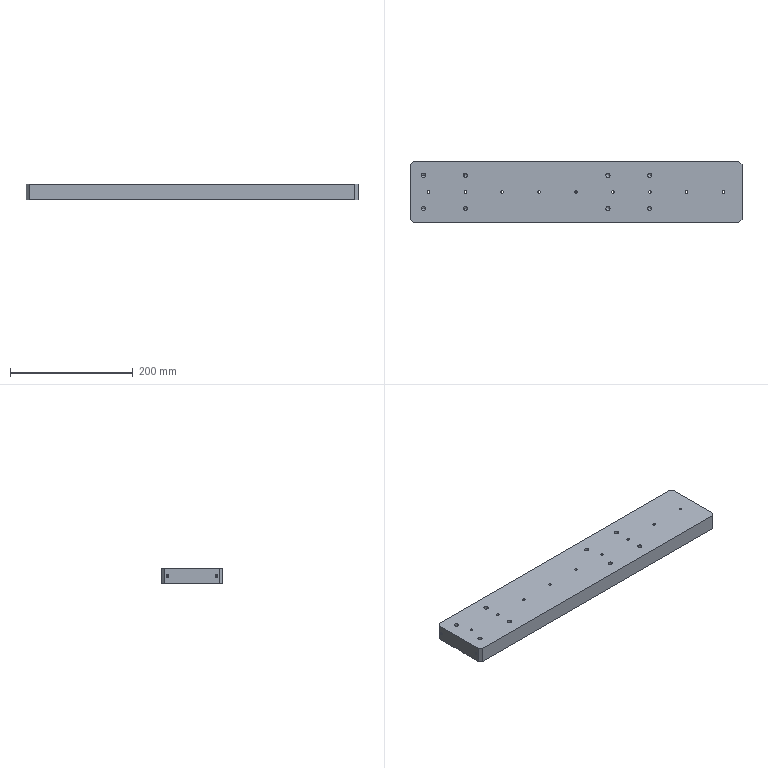Part | NX | features BREP 1 | 1 solid | 76 faces | box 540 x 100 x 26 mm | volume 1376932 mm3 | cylinder 40 | cone 22 | plane 14 | commonest cylinder face diameters 4.2 x24 6.8 x16